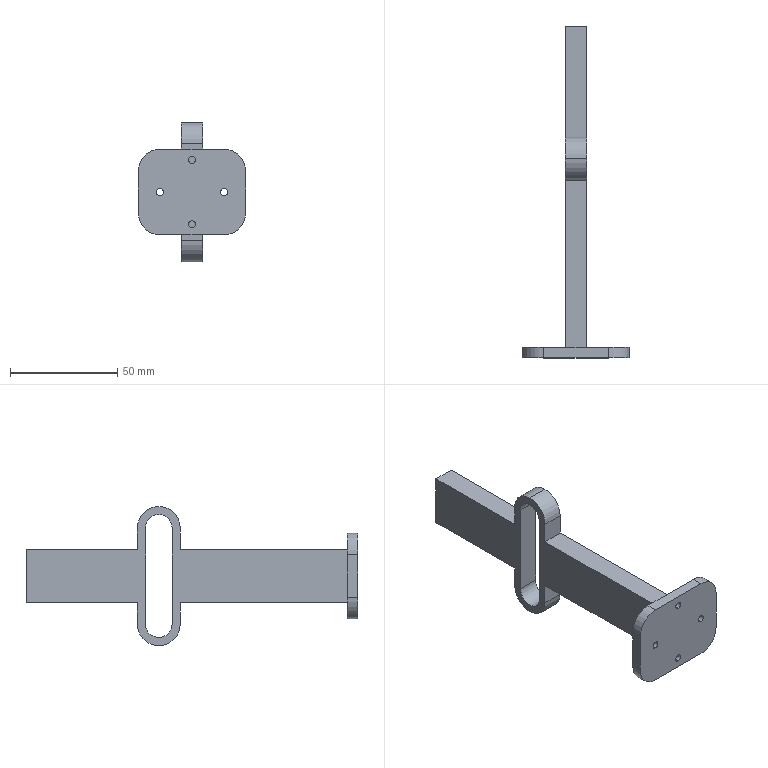Part | SolidWorks | features MirrorStock 1 | 1 solid | 37 faces | box 50 x 155 x 65 mm | volume 47254 mm3 | plane 19 | cylinder 18 | commonest cylinder face diameters 3.3 x8 20 x7 12.4 x3
STEP:
#1=CARTESIAN_POINT('',(15.,2.5,-1.65));
#2=VERTEX_POINT('',#1);
#3=CARTESIAN_POINT('',(15.,2.5,1.65));
#4=VERTEX_POINT('',#3);
#5=CARTESIAN_POINT('',(15.,2.5,0.));
#6=DIRECTION('',(0.,-1.,0.));
#7=DIRECTION('',(0.,0.,-1.));
#8=AXIS2_PLACEMENT_3D('',#5,#6,#7);
#9=CIRCLE('',#8,1.65);
#10=EDGE_CURVE('',#2,#4,#9,.T.);
#11=ORIENTED_EDGE('',*,*,#10,.F.);
#12=CARTESIAN_POINT('',(15.,-2.5,-1.65));
#13=VERTEX_POINT('',#12);
#14=CARTESIAN_POINT('',(15.,32.5,-1.65));
#15=DIRECTION('',(0.,-1.,0.));
#16=VECTOR('',#15,1000.);
#17=LINE('',#14,#16);
#18=EDGE_CURVE('',#2,#13,#17,.T.);
#19=ORIENTED_EDGE('',*,*,#18,.T.);
#20=CARTESIAN_POINT('',(15.,-2.5,1.65));
#21=VERTEX_POINT('',#20);
#22=CARTESIAN_POINT('',(15.,-2.5,0.));
#23=DIRECTION('',(0.,1.,0.));
#24=DIRECTION('',(0.,0.,1.));
#25=AXIS2_PLACEMENT_3D('',#22,#23,#24);
#26=CIRCLE('',#25,1.65);
#27=EDGE_CURVE('',#21,#13,#26,.T.);
#28=ORIENTED_EDGE('',*,*,#27,.F.);
#29=CARTESIAN_POINT('',(15.,32.5,1.65));
#30=DIRECTION('',(0.,-1.,0.));
#31=VECTOR('',#30,1000.);
#32=LINE('',#29,#31);
#33=EDGE_CURVE('',#4,#21,#32,.T.);
#34=ORIENTED_EDGE('',*,*,#33,.F.);
#35=EDGE_LOOP('',(#11,#19,#28,#34));
#36=FACE_OUTER_BOUND('',#35,.T.);
#37=CARTESIAN_POINT('',(15.,32.5,0.));
#38=DIRECTION('',(0.,-1.,0.));
#39=DIRECTION('',(0.,0.,1.));
#40=AXIS2_PLACEMENT_3D('',#37,#38,#39);
#41=CYLINDRICAL_SURFACE('',#40,1.65);
#42=ADVANCED_FACE('',(#36),#41,.F.);
#43=CARTESIAN_POINT('',(0.,2.5,13.35));
#44=VERTEX_POINT('',#43);
#45=CARTESIAN_POINT('',(0.,2.5,16.65));
#46=VERTEX_POINT('',#45);
#47=CARTESIAN_POINT('',(0.,2.5,15.));
#48=DIRECTION('',(0.,-1.,0.));
#49=DIRECTION('',(0.,0.,-1.));
#50=AXIS2_PLACEMENT_3D('',#47,#48,#49);
#51=CIRCLE('',#50,1.65);
#52=EDGE_CURVE('',#44,#46,#51,.T.);
#53=ORIENTED_EDGE('',*,*,#52,.F.);
#54=CARTESIAN_POINT('',(0.,-2.5,13.35));
#55=VERTEX_POINT('',#54);
#56=CARTESIAN_POINT('',(0.,32.5,13.35));
#57=DIRECTION('',(0.,-1.,0.));
#58=VECTOR('',#57,1000.);
#59=LINE('',#56,#58);
#60=EDGE_CURVE('',#44,#55,#59,.T.);
#61=ORIENTED_EDGE('',*,*,#60,.T.);
#62=CARTESIAN_POINT('',(0.,-2.5,16.65));
#63=VERTEX_POINT('',#62);
#64=CARTESIAN_POINT('',(0.,-2.5,15.));
#65=DIRECTION('',(0.,1.,0.));
#66=DIRECTION('',(0.,0.,1.));
#67=AXIS2_PLACEMENT_3D('',#64,#65,#66);
#68=CIRCLE('',#67,1.65);
#69=EDGE_CURVE('',#63,#55,#68,.T.);
#70=ORIENTED_EDGE('',*,*,#69,.F.);
#71=CARTESIAN_POINT('',(0.,32.5,16.65));
#72=DIRECTION('',(0.,-1.,0.));
#73=VECTOR('',#72,1000.);
#74=LINE('',#71,#73);
#75=EDGE_CURVE('',#46,#63,#74,.T.);
#76=ORIENTED_EDGE('',*,*,#75,.F.);
#77=EDGE_LOOP('',(#53,#61,#70,#76));
#78=FACE_OUTER_BOUND('',#77,.T.);
#79=CARTESIAN_POINT('',(0.,32.5,15.));
#80=DIRECTION('',(0.,-1.,0.));
#81=DIRECTION('',(0.,0.,1.));
#82=AXIS2_PLACEMENT_3D('',#79,#80,#81);
#83=CYLINDRICAL_SURFACE('',#82,1.65);
#84=ADVANCED_FACE('',(#78),#83,.F.);
#85=CARTESIAN_POINT('',(0.,2.5,-16.65));
#86=VERTEX_POINT('',#85);
#87=CARTESIAN_POINT('',(0.,2.5,-13.35));
#88=VERTEX_POINT('',#87);
#89=CARTESIAN_POINT('',(0.,2.5,-15.));
#90=DIRECTION('',(0.,-1.,0.));
#91=DIRECTION('',(0.,0.,-1.));
#92=AXIS2_PLACEMENT_3D('',#89,#90,#91);
#93=CIRCLE('',#92,1.65);
#94=EDGE_CURVE('',#86,#88,#93,.T.);
#95=ORIENTED_EDGE('',*,*,#94,.F.);
#96=CARTESIAN_POINT('',(0.,-2.5,-16.65));
#97=VERTEX_POINT('',#96);
#98=CARTESIAN_POINT('',(0.,32.5,-16.65));
#99=DIRECTION('',(0.,-1.,0.));
#100=VECTOR('',#99,1000.);
#101=LINE('',#98,#100);
#102=EDGE_CURVE('',#86,#97,#101,.T.);
#103=ORIENTED_EDGE('',*,*,#102,.T.);
#104=CARTESIAN_POINT('',(0.,-2.5,-13.35));
#105=VERTEX_POINT('',#104);
#106=CARTESIAN_POINT('',(0.,-2.5,-15.));
#107=DIRECTION('',(0.,1.,0.));
#108=DIRECTION('',(0.,0.,1.));
#109=AXIS2_PLACEMENT_3D('',#106,#107,#108);
#110=CIRCLE('',#109,1.65);
#111=EDGE_CURVE('',#105,#97,#110,.T.);
#112=ORIENTED_EDGE('',*,*,#111,.F.);
#113=CARTESIAN_POINT('',(0.,32.5,-13.35));
#114=DIRECTION('',(0.,-1.,0.));
#115=VECTOR('',#114,1000.);
#116=LINE('',#113,#115);
#117=EDGE_CURVE('',#88,#105,#116,.T.);
#118=ORIENTED_EDGE('',*,*,#117,.F.);
#119=EDGE_LOOP('',(#95,#103,#112,#118));
#120=FACE_OUTER_BOUND('',#119,.T.);
#121=CARTESIAN_POINT('',(0.,32.5,-15.));
#122=DIRECTION('',(0.,-1.,0.));
#123=DIRECTION('',(0.,0.,1.));
#124=AXIS2_PLACEMENT_3D('',#121,#122,#123);
#125=CYLINDRICAL_SURFACE('',#124,1.65);
#126=ADVANCED_FACE('',(#120),#125,.F.);
#127=CARTESIAN_POINT('',(-15.,2.5,-1.65));
#128=VERTEX_POINT('',#127);
#129=CARTESIAN_POINT('',(-15.,2.5,1.65));
#130=VERTEX_POINT('',#129);
#131=CARTESIAN_POINT('',(-15.,2.5,0.));
#132=DIRECTION('',(0.,-1.,0.));
#133=DIRECTION('',(0.,0.,-1.));
#134=AXIS2_PLACEMENT_3D('',#131,#132,#133);
#135=CIRCLE('',#134,1.65);
#136=EDGE_CURVE('',#128,#130,#135,.T.);
#137=ORIENTED_EDGE('',*,*,#136,.F.);
#138=CARTESIAN_POINT('',(-15.,-2.5,-1.65));
#139=VERTEX_POINT('',#138);
#140=CARTESIAN_POINT('',(-15.,32.5,-1.65));
#141=DIRECTION('',(0.,-1.,0.));
#142=VECTOR('',#141,1000.);
#143=LINE('',#140,#142);
#144=EDGE_CURVE('',#128,#139,#143,.T.);
#145=ORIENTED_EDGE('',*,*,#144,.T.);
#146=CARTESIAN_POINT('',(-15.,-2.5,1.65));
#147=VERTEX_POINT('',#146);
#148=CARTESIAN_POINT('',(-15.,-2.5,0.));
#149=DIRECTION('',(0.,1.,0.));
#150=DIRECTION('',(0.,0.,1.));
#151=AXIS2_PLACEMENT_3D('',#148,#149,#150);
#152=CIRCLE('',#151,1.65);
#153=EDGE_CURVE('',#147,#139,#152,.T.);
#154=ORIENTED_EDGE('',*,*,#153,.F.);
#155=CARTESIAN_POINT('',(-15.,32.5,1.65));
#156=DIRECTION('',(0.,-1.,0.));
#157=VECTOR('',#156,1000.);
#158=LINE('',#155,#157);
#159=EDGE_CURVE('',#130,#147,#158,.T.);
#160=ORIENTED_EDGE('',*,*,#159,.F.);
#161=EDGE_LOOP('',(#137,#145,#154,#160));
#162=FACE_OUTER_BOUND('',#161,.T.);
#163=CARTESIAN_POINT('',(-15.,32.5,0.));
#164=DIRECTION('',(0.,-1.,0.));
#165=DIRECTION('',(0.,0.,1.));
#166=AXIS2_PLACEMENT_3D('',#163,#164,#165);
#167=CYLINDRICAL_SURFACE('',#166,1.65);
#168=ADVANCED_FACE('',(#162),#167,.F.);
#169=CARTESIAN_POINT('',(-5.,84.3,22.5));
#170=VERTEX_POINT('',#169);
#171=CARTESIAN_POINT('',(-5.,90.5,28.7));
#172=VERTEX_POINT('',#171);
#173=CARTESIAN_POINT('',(-5.,90.5,22.5));
#174=DIRECTION('',(-1.,0.,0.));
#175=DIRECTION('',(0.,0.,1.));
#176=AXIS2_PLACEMENT_3D('',#173,#174,#175);
#177=CIRCLE('',#176,6.2);
#178=EDGE_CURVE('',#170,#172,#177,.T.);
#179=ORIENTED_EDGE('',*,*,#178,.T.);
#180=CARTESIAN_POINT('',(5.,90.5,28.7));
#181=VERTEX_POINT('',#180);
#182=CARTESIAN_POINT('',(-45.,90.5,28.7));
#183=DIRECTION('',(1.,0.,0.));
#184=VECTOR('',#183,1000.);
#185=LINE('',#182,#184);
#186=EDGE_CURVE('',#172,#181,#185,.T.);
#187=ORIENTED_EDGE('',*,*,#186,.T.);
#188=CARTESIAN_POINT('',(5.,84.3,22.5));
#189=VERTEX_POINT('',#188);
#190=CARTESIAN_POINT('',(5.,90.5,22.5));
#191=DIRECTION('',(-1.,0.,0.));
#192=DIRECTION('',(0.,0.,1.));
#193=AXIS2_PLACEMENT_3D('',#190,#191,#192);
#194=CIRCLE('',#193,6.2);
#195=EDGE_CURVE('',#189,#181,#194,.T.);
#196=ORIENTED_EDGE('',*,*,#195,.F.);
#197=CARTESIAN_POINT('',(-45.,84.3,22.5));
#198=DIRECTION('',(1.,0.,0.));
#199=VECTOR('',#198,1000.);
#200=LINE('',#197,#199);
#201=EDGE_CURVE('',#170,#189,#200,.T.);
#202=ORIENTED_EDGE('',*,*,#201,.F.);
#203=EDGE_LOOP('',(#179,#187,#196,#202));
#204=FACE_OUTER_BOUND('',#203,.T.);
#205=CARTESIAN_POINT('',(-45.,90.5,22.5));
#206=DIRECTION('',(1.,0.,0.));
#207=DIRECTION('',(0.,0.,1.));
#208=AXIS2_PLACEMENT_3D('',#205,#206,#207);
#209=CYLINDRICAL_SURFACE('',#208,6.2);
#210=ADVANCED_FACE('',(#204),#209,.F.);
#211=CARTESIAN_POINT('',(-5.,100.5,22.5));
#212=VERTEX_POINT('',#211);
#213=CARTESIAN_POINT('',(-5.,90.5,32.5));
#214=VERTEX_POINT('',#213);
#215=CARTESIAN_POINT('',(-5.,90.5,22.5));
#216=DIRECTION('',(1.,0.,0.));
#217=DIRECTION('',(0.,0.,1.));
#218=AXIS2_PLACEMENT_3D('',#215,#216,#217);
#219=CIRCLE('',#218,10.);
#220=EDGE_CURVE('',#212,#214,#219,.T.);
#221=ORIENTED_EDGE('',*,*,#220,.T.);
#222=CARTESIAN_POINT('',(5.,90.5,32.5));
#223=VERTEX_POINT('',#222);
#224=CARTESIAN_POINT('',(-73.007,90.5,32.5));
#225=DIRECTION('',(1.,0.,0.));
#226=VECTOR('',#225,1000.);
#227=LINE('',#224,#226);
#228=EDGE_CURVE('',#214,#223,#227,.T.);
#229=ORIENTED_EDGE('',*,*,#228,.T.);
#230=CARTESIAN_POINT('',(5.,100.5,22.5));
#231=VERTEX_POINT('',#230);
#232=CARTESIAN_POINT('',(5.,90.5,22.5));
#233=DIRECTION('',(-1.,0.,0.));
#234=DIRECTION('',(0.,0.,1.));
#235=AXIS2_PLACEMENT_3D('',#232,#233,#234);
#236=CIRCLE('',#235,10.);
#237=EDGE_CURVE('',#223,#231,#236,.T.);
#238=ORIENTED_EDGE('',*,*,#237,.T.);
#239=CARTESIAN_POINT('',(-73.007,100.5,22.5));
#240=DIRECTION('',(1.,0.,0.));
#241=VECTOR('',#240,1000.);
#242=LINE('',#239,#241);
#243=EDGE_CURVE('',#212,#231,#242,.T.);
#244=ORIENTED_EDGE('',*,*,#243,.F.);
#245=EDGE_LOOP('',(#221,#229,#238,#244));
#246=FACE_OUTER_BOUND('',#245,.T.);
#247=CARTESIAN_POINT('',(-73.007,90.5,22.5));
#248=DIRECTION('',(1.,0.,0.));
#249=DIRECTION('',(0.,0.,1.));
#250=AXIS2_PLACEMENT_3D('',#247,#248,#249);
#251=CYLINDRICAL_SURFACE('',#250,10.);
#252=ADVANCED_FACE('',(#246),#251,.T.);
#253=CARTESIAN_POINT('',(5.,152.5,12.5));
#254=VERTEX_POINT('',#253);
#255=CARTESIAN_POINT('',(5.,100.5,12.5));
#256=VERTEX_POINT('',#255);
#257=CARTESIAN_POINT('',(5.,152.5,12.5));
#258=DIRECTION('',(0.,-1.,0.));
#259=VECTOR('',#258,1000.);
#260=LINE('',#257,#259);
#261=EDGE_CURVE('',#254,#256,#260,.T.);
#262=ORIENTED_EDGE('',*,*,#261,.F.);
#263=CARTESIAN_POINT('',(-5.,152.5,12.5));
#264=VERTEX_POINT('',#263);
#265=CARTESIAN_POINT('',(-5.,152.5,12.5));
#266=DIRECTION('',(-1.,0.,0.));
#267=VECTOR('',#266,1000.);
#268=LINE('',#265,#267);
#269=EDGE_CURVE('',#254,#264,#268,.T.);
#270=ORIENTED_EDGE('',*,*,#269,.T.);
#271=CARTESIAN_POINT('',(-5.,100.5,12.5));
#272=VERTEX_POINT('',#271);
#273=CARTESIAN_POINT('',(-5.,152.5,12.5));
#274=DIRECTION('',(0.,-1.,0.));
#275=VECTOR('',#274,1000.);
#276=LINE('',#273,#275);
#277=EDGE_CURVE('',#264,#272,#276,.T.);
#278=ORIENTED_EDGE('',*,*,#277,.T.);
#279=CARTESIAN_POINT('',(-5.,100.5,12.5));
#280=DIRECTION('',(-1.,0.,0.));
#281=VECTOR('',#280,1000.);
#282=LINE('',#279,#281);
#283=EDGE_CURVE('',#256,#272,#282,.T.);
#284=ORIENTED_EDGE('',*,*,#283,.F.);
#285=EDGE_LOOP('',(#262,#270,#278,#284));
#286=FACE_OUTER_BOUND('',#285,.T.);
#287=CARTESIAN_POINT('',(-5.,152.5,12.5));
#288=DIRECTION('',(0.,0.,-1.));
#289=DIRECTION('',(1.,0.,0.));
#290=AXIS2_PLACEMENT_3D('',#287,#288,#289);
#291=PLANE('',#290);
#292=ADVANCED_FACE('',(#286),#291,.F.);
#293=CARTESIAN_POINT('',(-5.,152.5,-12.5));
#294=VERTEX_POINT('',#293);
#295=CARTESIAN_POINT('',(-5.,100.5,-12.5));
#296=VERTEX_POINT('',#295);
#297=CARTESIAN_POINT('',(-5.,152.5,-12.5));
#298=DIRECTION('',(0.,-1.,0.));
#299=VECTOR('',#298,1000.);
#300=LINE('',#297,#299);
#301=EDGE_CURVE('',#294,#296,#300,.T.);
#302=ORIENTED_EDGE('',*,*,#301,.F.);
#303=CARTESIAN_POINT('',(5.,152.5,-12.5));
#304=VERTEX_POINT('',#303);
#305=CARTESIAN_POINT('',(-5.,152.5,-12.5));
#306=DIRECTION('',(1.,0.,0.));
#307=VECTOR('',#306,1000.);
#308=LINE('',#305,#307);
#309=EDGE_CURVE('',#294,#304,#308,.T.);
#310=ORIENTED_EDGE('',*,*,#309,.T.);
#311=CARTESIAN_POINT('',(5.,100.5,-12.5));
#312=VERTEX_POINT('',#311);
#313=CARTESIAN_POINT('',(5.,152.5,-12.5));
#314=DIRECTION('',(0.,-1.,0.));
#315=VECTOR('',#314,1000.);
#316=LINE('',#313,#315);
#317=EDGE_CURVE('',#304,#312,#316,.T.);
#318=ORIENTED_EDGE('',*,*,#317,.T.);
#319=CARTESIAN_POINT('',(-5.,100.5,-12.5));
#320=DIRECTION('',(1.,0.,0.));
#321=VECTOR('',#320,1000.);
#322=LINE('',#319,#321);
#323=EDGE_CURVE('',#296,#312,#322,.T.);
#324=ORIENTED_EDGE('',*,*,#323,.F.);
#325=EDGE_LOOP('',(#302,#310,#318,#324));
#326=FACE_OUTER_BOUND('',#325,.T.);
#327=CARTESIAN_POINT('',(-5.,152.5,-12.5));
#328=DIRECTION('',(0.,0.,1.));
#329=DIRECTION('',(-1.,0.,0.));
#330=AXIS2_PLACEMENT_3D('',#327,#328,#329);
#331=PLANE('',#330);
#332=ADVANCED_FACE('',(#326),#331,.F.);
#333=ORIENTED_EDGE('',*,*,#27,.T.);
#334=CARTESIAN_POINT('',(15.,-2.5,0.));
#335=DIRECTION('',(0.,1.,0.));
#336=DIRECTION('',(0.,0.,1.));
#337=AXIS2_PLACEMENT_3D('',#334,#335,#336);
#338=CIRCLE('',#337,1.65);
#339=EDGE_CURVE('',#13,#21,#338,.T.);
#340=ORIENTED_EDGE('',*,*,#339,.T.);
#341=EDGE_LOOP('',(#333,#340));
#342=FACE_BOUND('',#341,.T.);
#343=ORIENTED_EDGE('',*,*,#69,.T.);
#344=CARTESIAN_POINT('',(0.,-2.5,15.));
#345=DIRECTION('',(0.,1.,0.));
#346=DIRECTION('',(0.,0.,1.));
#347=AXIS2_PLACEMENT_3D('',#344,#345,#346);
#348=CIRCLE('',#347,1.65);
#349=EDGE_CURVE('',#55,#63,#348,.T.);
#350=ORIENTED_EDGE('',*,*,#349,.T.);
#351=EDGE_LOOP('',(#343,#350));
#352=FACE_BOUND('',#351,.T.);
#353=ORIENTED_EDGE('',*,*,#111,.T.);
#354=CARTESIAN_POINT('',(0.,-2.5,-15.));
#355=DIRECTION('',(0.,1.,0.));
#356=DIRECTION('',(0.,0.,1.));
#357=AXIS2_PLACEMENT_3D('',#354,#355,#356);
#358=CIRCLE('',#357,1.65);
#359=EDGE_CURVE('',#97,#105,#358,.T.);
#360=ORIENTED_EDGE('',*,*,#359,.T.);
#361=EDGE_LOOP('',(#353,#360));
#362=FACE_BOUND('',#361,.T.);
#363=ORIENTED_EDGE('',*,*,#153,.T.);
#364=CARTESIAN_POINT('',(-15.,-2.5,0.));
#365=DIRECTION('',(0.,1.,0.));
#366=DIRECTION('',(0.,0.,1.));
#367=AXIS2_PLACEMENT_3D('',#364,#365,#366);
#368=CIRCLE('',#367,1.65);
#369=EDGE_CURVE('',#139,#147,#368,.T.);
#370=ORIENTED_EDGE('',*,*,#369,.T.);
#371=EDGE_LOOP('',(#363,#370));
#372=FACE_BOUND('',#371,.T.);
#373=CARTESIAN_POINT('',(-25.,-2.5,-10.));
#374=VERTEX_POINT('',#373);
#375=CARTESIAN_POINT('',(-25.,-2.5,10.));
#376=VERTEX_POINT('',#375);
#377=CARTESIAN_POINT('',(-25.,-2.5,-20.));
#378=DIRECTION('',(0.,0.,1.));
#379=VECTOR('',#378,1000.);
#380=LINE('',#377,#379);
#381=EDGE_CURVE('',#374,#376,#380,.T.);
#382=ORIENTED_EDGE('',*,*,#381,.F.);
#383=CARTESIAN_POINT('',(-15.,-2.5,-20.));
#384=VERTEX_POINT('',#383);
#385=CARTESIAN_POINT('',(-15.,-2.5,-10.));
#386=DIRECTION('',(0.,1.,0.));
#387=DIRECTION('',(0.,0.,-1.));
#388=AXIS2_PLACEMENT_3D('',#385,#386,#387);
#389=CIRCLE('',#388,10.);
#390=EDGE_CURVE('',#384,#374,#389,.T.);
#391=ORIENTED_EDGE('',*,*,#390,.F.);
#392=CARTESIAN_POINT('',(15.,-2.5,-20.));
#393=VERTEX_POINT('',#392);
#394=CARTESIAN_POINT('',(0.,-2.5,-20.));
#395=DIRECTION('',(1.,0.,0.));
#396=VECTOR('',#395,1000.);
#397=LINE('',#394,#396);
#398=EDGE_CURVE('',#384,#393,#397,.T.);
#399=ORIENTED_EDGE('',*,*,#398,.T.);
#400=CARTESIAN_POINT('',(25.,-2.5,-10.));
#401=VERTEX_POINT('',#400);
#402=CARTESIAN_POINT('',(15.,-2.5,-10.));
#403=DIRECTION('',(0.,1.,0.));
#404=DIRECTION('',(0.,0.,-1.));
#405=AXIS2_PLACEMENT_3D('',#402,#403,#404);
#406=CIRCLE('',#405,10.);
#407=EDGE_CURVE('',#401,#393,#406,.T.);
#408=ORIENTED_EDGE('',*,*,#407,.F.);
#409=CARTESIAN_POINT('',(25.,-2.5,10.));
#410=VERTEX_POINT('',#409);
#411=CARTESIAN_POINT('',(25.,-2.5,-20.));
#412=DIRECTION('',(0.,0.,1.));
#413=VECTOR('',#412,1000.);
#414=LINE('',#411,#413);
#415=EDGE_CURVE('',#401,#410,#414,.T.);
#416=ORIENTED_EDGE('',*,*,#415,.T.);
#417=CARTESIAN_POINT('',(15.,-2.5,20.));
#418=VERTEX_POINT('',#417);
#419=CARTESIAN_POINT('',(15.,-2.5,10.));
#420=DIRECTION('',(0.,1.,0.));
#421=DIRECTION('',(0.,0.,-1.));
#422=AXIS2_PLACEMENT_3D('',#419,#420,#421);
#423=CIRCLE('',#422,10.);
#424=EDGE_CURVE('',#418,#410,#423,.T.);
#425=ORIENTED_EDGE('',*,*,#424,.F.);
#426=CARTESIAN_POINT('',(-15.,-2.5,20.));
#427=VERTEX_POINT('',#426);
#428=CARTESIAN_POINT('',(0.,-2.5,20.));
#429=DIRECTION('',(1.,0.,0.));
#430=VECTOR('',#429,1000.);
#431=LINE('',#428,#430);
#432=EDGE_CURVE('',#427,#418,#431,.T.);
#433=ORIENTED_EDGE('',*,*,#432,.F.);
#434=CARTESIAN_POINT('',(-15.,-2.5,10.));
#435=DIRECTION('',(0.,1.,0.));
#436=DIRECTION('',(0.,0.,-1.));
#437=AXIS2_PLACEMENT_3D('',#434,#435,#436);
#438=CIRCLE('',#437,10.);
#439=EDGE_CURVE('',#376,#427,#438,.T.);
#440=ORIENTED_EDGE('',*,*,#439,.F.);
#441=EDGE_LOOP('',(#382,#391,#399,#408,#416,#425,#433,#440));
#442=FACE_OUTER_BOUND('',#441,.T.);
#443=CARTESIAN_POINT('',(0.,-2.5,-20.));
#444=DIRECTION('',(0.,1.,0.));
#445=DIRECTION('',(0.,0.,-1.));
#446=AXIS2_PLACEMENT_3D('',#443,#444,#445);
#447=PLANE('',#446);
#448=ADVANCED_FACE('',(#342,#352,#362,#372,#442),#447,.F.);
#449=ORIENTED_EDGE('',*,*,#415,.F.);
#450=CARTESIAN_POINT('',(25.,2.5,-10.));
#451=VERTEX_POINT('',#450);
#452=CARTESIAN_POINT('',(25.,-2.5,-10.));
#453=DIRECTION('',(0.,-1.,0.));
#454=VECTOR('',#453,1000.);
#455=LINE('',#452,#454);
#456=EDGE_CURVE('',#451,#401,#455,.T.);
#457=ORIENTED_EDGE('',*,*,#456,.F.);
#458=CARTESIAN_POINT('',(25.,2.5,10.));
#459=VERTEX_POINT('',#458);
#460=CARTESIAN_POINT('',(25.,2.5,-20.));
#461=DIRECTION('',(0.,0.,1.));
#462=VECTOR('',#461,1000.);
#463=LINE('',#460,#462);
#464=EDGE_CURVE('',#451,#459,#463,.T.);
#465=ORIENTED_EDGE('',*,*,#464,.T.);
#466=CARTESIAN_POINT('',(25.,0.,10.));
#467=DIRECTION('',(0.,1.,0.));
#468=VECTOR('',#467,1000.);
#469=LINE('',#466,#468);
#470=EDGE_CURVE('',#410,#459,#469,.T.);
#471=ORIENTED_EDGE('',*,*,#470,.F.);
#472=EDGE_LOOP('',(#449,#457,#465,#471));
#473=FACE_OUTER_BOUND('',#472,.T.);
#474=CARTESIAN_POINT('',(25.,0.,-20.));
#475=DIRECTION('',(-1.,0.,0.));
#476=DIRECTION('',(0.,0.,-1.));
#477=AXIS2_PLACEMENT_3D('',#474,#475,#476);
#478=PLANE('',#477);
#479=ADVANCED_FACE('',(#473),#478,.F.);
#480=CARTESIAN_POINT('',(15.,2.5,0.));
#481=DIRECTION('',(0.,-1.,0.));
#482=DIRECTION('',(0.,0.,-1.));
#483=AXIS2_PLACEMENT_3D('',#480,#481,#482);
#484=CIRCLE('',#483,1.65);
#485=EDGE_CURVE('',#4,#2,#484,.T.);
#486=ORIENTED_EDGE('',*,*,#485,.T.);
#487=ORIENTED_EDGE('',*,*,#10,.T.);
#488=EDGE_LOOP('',(#486,#487));
#489=FACE_BOUND('',#488,.T.);
#490=CARTESIAN_POINT('',(0.,2.5,15.));
#491=DIRECTION('',(0.,-1.,0.));
#492=DIRECTION('',(0.,0.,-1.));
#493=AXIS2_PLACEMENT_3D('',#490,#491,#492);
#494=CIRCLE('',#493,1.65);
#495=EDGE_CURVE('',#46,#44,#494,.T.);
#496=ORIENTED_EDGE('',*,*,#495,.T.);
#497=ORIENTED_EDGE('',*,*,#52,.T.);
#498=EDGE_LOOP('',(#496,#497));
#499=FACE_BOUND('',#498,.T.);
#500=CARTESIAN_POINT('',(0.,2.5,-15.));
#501=DIRECTION('',(0.,-1.,0.));
#502=DIRECTION('',(0.,0.,-1.));
#503=AXIS2_PLACEMENT_3D('',#500,#501,#502);
#504=CIRCLE('',#503,1.65);
#505=EDGE_CURVE('',#88,#86,#504,.T.);
#506=ORIENTED_EDGE('',*,*,#505,.T.);
#507=ORIENTED_EDGE('',*,*,#94,.T.);
#508=EDGE_LOOP('',(#506,#507));
#509=FACE_BOUND('',#508,.T.);
#510=CARTESIAN_POINT('',(-15.,2.5,0.));
#511=DIRECTION('',(0.,-1.,0.));
#512=DIRECTION('',(0.,0.,-1.));
#513=AXIS2_PLACEMENT_3D('',#510,#511,#512);
#514=CIRCLE('',#513,1.65);
#515=EDGE_CURVE('',#130,#128,#514,.T.);
#516=ORIENTED_EDGE('',*,*,#515,.T.);
#517=ORIENTED_EDGE('',*,*,#136,.T.);
#518=EDGE_LOOP('',(#516,#517));
#519=FACE_BOUND('',#518,.T.);
#520=CARTESIAN_POINT('',(5.,2.5,-12.5));
#521=VERTEX_POINT('',#520);
#522=CARTESIAN_POINT('',(5.,2.5,12.5));
#523=VERTEX_POINT('',#522);
#524=CARTESIAN_POINT('',(5.,2.5,-12.5));
#525=DIRECTION('',(0.,0.,1.));
#526=VECTOR('',#525,1000.);
#527=LINE('',#524,#526);
#528=EDGE_CURVE('',#521,#523,#527,.T.);
#529=ORIENTED_EDGE('',*,*,#528,.T.);
#530=CARTESIAN_POINT('',(-5.,2.5,12.5));
#531=VERTEX_POINT('',#530);
#532=CARTESIAN_POINT('',(-5.,2.5,12.5));
#533=DIRECTION('',(-1.,0.,0.));
#534=VECTOR('',#533,1000.);
#535=LINE('',#532,#534);
#536=EDGE_CURVE('',#523,#531,#535,.T.);
#537=ORIENTED_EDGE('',*,*,#536,.T.);
#538=CARTESIAN_POINT('',(-5.,2.5,-12.5));
#539=VERTEX_POINT('',#538);
#540=CARTESIAN_POINT('',(-5.,2.5,-12.5));
#541=DIRECTION('',(0.,0.,-1.));
#542=VECTOR('',#541,1000.);
#543=LINE('',#540,#542);
#544=EDGE_CURVE('',#531,#539,#543,.T.);
#545=ORIENTED_EDGE('',*,*,#544,.T.);
#546=CARTESIAN_POINT('',(-5.,2.5,-12.5));
#547=DIRECTION('',(1.,0.,0.));
#548=VECTOR('',#547,1000.);
#549=LINE('',#546,#548);
#550=EDGE_CURVE('',#539,#521,#549,.T.);
#551=ORIENTED_EDGE('',*,*,#550,.T.);
#552=EDGE_LOOP('',(#529,#537,#545,#551));
#553=FACE_BOUND('',#552,.T.);
#554=CARTESIAN_POINT('',(-15.,2.5,20.));
#555=VERTEX_POINT('',#554);
#556=CARTESIAN_POINT('',(15.,2.5,20.));
#557=VERTEX_POINT('',#556);
#558=CARTESIAN_POINT('',(0.,2.5,20.));
#559=DIRECTION('',(1.,0.,0.));
#560=VECTOR('',#559,1000.);
#561=LINE('',#558,#560);
#562=EDGE_CURVE('',#555,#557,#561,.T.);
#563=ORIENTED_EDGE('',*,*,#562,.T.);
#564=CARTESIAN_POINT('',(15.,2.5,10.));
#565=DIRECTION('',(0.,-1.,0.));
#566=DIRECTION('',(0.,0.,-1.));
#567=AXIS2_PLACEMENT_3D('',#564,#565,#566);
#568=CIRCLE('',#567,10.);
#569=EDGE_CURVE('',#459,#557,#568,.T.);
#570=ORIENTED_EDGE('',*,*,#569,.F.);
#571=ORIENTED_EDGE('',*,*,#464,.F.);
#572=CARTESIAN_POINT('',(15.,2.5,-20.));
#573=VERTEX_POINT('',#572);
#574=CARTESIAN_POINT('',(15.,2.5,-10.));
#575=DIRECTION('',(0.,-1.,0.));
#576=DIRECTION('',(0.,0.,-1.));
#577=AXIS2_PLACEMENT_3D('',#574,#575,#576);
#578=CIRCLE('',#577,10.);
#579=EDGE_CURVE('',#573,#451,#578,.T.);
#580=ORIENTED_EDGE('',*,*,#579,.F.);
#581=CARTESIAN_POINT('',(-15.,2.5,-20.));
#582=VERTEX_POINT('',#581);
#583=CARTESIAN_POINT('',(0.,2.5,-20.));
#584=DIRECTION('',(1.,0.,0.));
#585=VECTOR('',#584,1000.);
#586=LINE('',#583,#585);
#587=EDGE_CURVE('',#582,#573,#586,.T.);
#588=ORIENTED_EDGE('',*,*,#587,.F.);
#589=CARTESIAN_POINT('',(-25.,2.5,-10.));
#590=VERTEX_POINT('',#589);
#591=CARTESIAN_POINT('',(-15.,2.5,-10.));
#592=DIRECTION('',(0.,-1.,0.));
#593=DIRECTION('',(0.,0.,-1.));
#594=AXIS2_PLACEMENT_3D('',#591,#592,#593);
#595=CIRCLE('',#594,10.);
#596=EDGE_CURVE('',#590,#582,#595,.T.);
#597=ORIENTED_EDGE('',*,*,#596,.F.);
#598=CARTESIAN_POINT('',(-25.,2.5,10.));
#599=VERTEX_POINT('',#598);
#600=CARTESIAN_POINT('',(-25.,2.5,-20.));
#601=DIRECTION('',(0.,0.,1.));
#602=VECTOR('',#601,1000.);
#603=LINE('',#600,#602);
#604=EDGE_CURVE('',#590,#599,#603,.T.);
#605=ORIENTED_EDGE('',*,*,#604,.T.);
#606=CARTESIAN_POINT('',(-15.,2.5,10.));
#607=DIRECTION('',(0.,-1.,0.));
#608=DIRECTION('',(0.,0.,-1.));
#609=AXIS2_PLACEMENT_3D('',#606,#607,#608);
#610=CIRCLE('',#609,10.);
#611=EDGE_CURVE('',#555,#599,#610,.T.);
#612=ORIENTED_EDGE('',*,*,#611,.F.);
#613=EDGE_LOOP('',(#563,#570,#571,#580,#588,#597,#605,#612));
#614=FACE_OUTER_BOUND('',#613,.T.);
#615=CARTESIAN_POINT('',(0.,2.5,-20.));
#616=DIRECTION('',(0.,1.,0.));
#617=DIRECTION('',(0.,0.,-1.));
#618=AXIS2_PLACEMENT_3D('',#615,#616,#617);
#619=PLANE('',#618);
#620=ADVANCED_FACE('',(#489,#499,#509,#519,#553,#614),#619,.T.);
#621=ORIENTED_EDGE('',*,*,#604,.F.);
#622=CARTESIAN_POINT('',(-25.,0.,-10.));
#623=DIRECTION('',(0.,1.,0.));
#624=VECTOR('',#623,1000.);
#625=LINE('',#622,#624);
#626=EDGE_CURVE('',#374,#590,#625,.T.);
#627=ORIENTED_EDGE('',*,*,#626,.F.);
#628=ORIENTED_EDGE('',*,*,#381,.T.);
#629=CARTESIAN_POINT('',(-25.,-2.5,10.));
#630=DIRECTION('',(0.,-1.,0.));
#631=VECTOR('',#630,1000.);
#632=LINE('',#629,#631);
#633=EDGE_CURVE('',#599,#376,#632,.T.);
#634=ORIENTED_EDGE('',*,*,#633,.F.);
#635=EDGE_LOOP('',(#621,#627,#628,#634));
#636=FACE_OUTER_BOUND('',#635,.T.);
#637=CARTESIAN_POINT('',(-25.,0.,-20.));
#638=DIRECTION('',(-1.,0.,0.));
#639=DIRECTION('',(0.,0.,-1.));
#640=AXIS2_PLACEMENT_3D('',#637,#638,#639);
#641=PLANE('',#640);
#642=ADVANCED_FACE('',(#636),#641,.T.);
#643=ORIENTED_EDGE('',*,*,#398,.F.);
#644=CARTESIAN_POINT('',(-15.,0.,-20.));
#645=DIRECTION('',(0.,-1.,0.));
#646=VECTOR('',#645,1000.);
#647=LINE('',#644,#646);
#648=EDGE_CURVE('',#582,#384,#647,.T.);
#649=ORIENTED_EDGE('',*,*,#648,.F.);
#650=ORIENTED_EDGE('',*,*,#587,.T.);
#651=CARTESIAN_POINT('',(15.,2.5,-20.));
#652=DIRECTION('',(0.,1.,0.));
#653=VECTOR('',#652,1000.);
#654=LINE('',#651,#653);
#655=EDGE_CURVE('',#393,#573,#654,.T.);
#656=ORIENTED_EDGE('',*,*,#655,.F.);
#657=EDGE_LOOP('',(#643,#649,#650,#656));
#658=FACE_OUTER_BOUND('',#657,.T.);
#659=CARTESIAN_POINT('',(0.,0.,-20.));
#660=DIRECTION('',(0.,0.,-1.));
#661=DIRECTION('',(1.,0.,0.));
#662=AXIS2_PLACEMENT_3D('',#659,#660,#661);
#663=PLANE('',#662);
#664=ADVANCED_FACE('',(#658),#663,.T.);
#665=ORIENTED_EDGE('',*,*,#432,.T.);
#666=CARTESIAN_POINT('',(15.,0.,20.));
#667=DIRECTION('',(0.,-1.,0.));
#668=VECTOR('',#667,1000.);
#669=LINE('',#666,#668);
#670=EDGE_CURVE('',#557,#418,#669,.T.);
#671=ORIENTED_EDGE('',*,*,#670,.F.);
#672=ORIENTED_EDGE('',*,*,#562,.F.);
#673=CARTESIAN_POINT('',(-15.,2.5,20.));
#674=DIRECTION('',(0.,1.,0.));
#675=VECTOR('',#674,1000.);
#676=LINE('',#673,#675);
#677=EDGE_CURVE('',#427,#555,#676,.T.);
#678=ORIENTED_EDGE('',*,*,#677,.F.);
#679=EDGE_LOOP('',(#665,#671,#672,#678));
#680=FACE_OUTER_BOUND('',#679,.T.);
#681=CARTESIAN_POINT('',(0.,0.,20.));
#682=DIRECTION('',(0.,0.,-1.));
#683=DIRECTION('',(1.,0.,0.));
#684=AXIS2_PLACEMENT_3D('',#681,#682,#683);
#685=PLANE('',#684);
#686=ADVANCED_FACE('',(#680),#685,.F.);
#687=CARTESIAN_POINT('',(5.,96.7,-22.5));
#688=VERTEX_POINT('',#687);
#689=CARTESIAN_POINT('',(5.,84.3,-22.5));
#690=VERTEX_POINT('',#689);
#691=CARTESIAN_POINT('',(5.,90.5,-22.5));
#692=DIRECTION('',(-1.,0.,0.));
#693=DIRECTION('',(0.,0.,1.));
#694=AXIS2_PLACEMENT_3D('',#691,#692,#693);
#695=CIRCLE('',#694,6.2);
#696=EDGE_CURVE('',#688,#690,#695,.T.);
#697=ORIENTED_EDGE('',*,*,#696,.T.);
#698=CARTESIAN_POINT('',(5.,84.3,0.));
#699=DIRECTION('',(0.,0.,1.));
#700=VECTOR('',#699,1000.);
#701=LINE('',#698,#700);
#702=EDGE_CURVE('',#690,#189,#701,.T.);
#703=ORIENTED_EDGE('',*,*,#702,.T.);
#704=ORIENTED_EDGE('',*,*,#195,.T.);
#705=CARTESIAN_POINT('',(5.,96.7,22.5));
#706=VERTEX_POINT('',#705);
#707=CARTESIAN_POINT('',(5.,90.5,22.5));
#708=DIRECTION('',(-1.,0.,0.));
#709=DIRECTION('',(0.,0.,1.));
#710=AXIS2_PLACEMENT_3D('',#707,#708,#709);
#711=CIRCLE('',#710,6.2);
#712=EDGE_CURVE('',#181,#706,#711,.T.);
#713=ORIENTED_EDGE('',*,*,#712,.T.);
#714=CARTESIAN_POINT('',(5.,96.7,0.));
#715=DIRECTION('',(0.,0.,-1.));
#716=VECTOR('',#715,1000.);
#717=LINE('',#714,#716);
#718=EDGE_CURVE('',#706,#688,#717,.T.);
#719=ORIENTED_EDGE('',*,*,#718,.T.);
#720=EDGE_LOOP('',(#697,#703,#704,#713,#719));
#721=FACE_BOUND('',#720,.T.);
#722=CARTESIAN_POINT('',(5.,80.5,12.5));
#723=VERTEX_POINT('',#722);
#724=CARTESIAN_POINT('',(5.,152.5,12.5));
#725=DIRECTION('',(0.,-1.,0.));
#726=VECTOR('',#725,1000.);
#727=LINE('',#724,#726);
#728=EDGE_CURVE('',#723,#523,#727,.T.);
#729=ORIENTED_EDGE('',*,*,#728,.T.);
#730=ORIENTED_EDGE('',*,*,#528,.F.);
#731=CARTESIAN_POINT('',(5.,80.5,-12.5));
#732=VERTEX_POINT('',#731);
#733=CARTESIAN_POINT('',(5.,152.5,-12.5));
#734=DIRECTION('',(0.,-1.,0.));
#735=VECTOR('',#734,1000.);
#736=LINE('',#733,#735);
#737=EDGE_CURVE('',#732,#521,#736,.T.);
#738=ORIENTED_EDGE('',*,*,#737,.F.);
#739=CARTESIAN_POINT('',(5.,80.5,-22.5));
#740=VERTEX_POINT('',#739);
#741=CARTESIAN_POINT('',(5.,80.5,-22.5));
#742=DIRECTION('',(0.,0.,1.));
#743=VECTOR('',#742,1000.);
#744=LINE('',#741,#743);
#745=EDGE_CURVE('',#740,#732,#744,.T.);
#746=ORIENTED_EDGE('',*,*,#745,.F.);
#747=CARTESIAN_POINT('',(5.,100.5,-22.5));
#748=VERTEX_POINT('',#747);
#749=CARTESIAN_POINT('',(5.,90.5,-22.5));
#750=DIRECTION('',(-1.,0.,0.));
#751=DIRECTION('',(0.,0.,1.));
#752=AXIS2_PLACEMENT_3D('',#749,#750,#751);
#753=CIRCLE('',#752,10.);
#754=EDGE_CURVE('',#748,#740,#753,.T.);
#755=ORIENTED_EDGE('',*,*,#754,.F.);
#756=CARTESIAN_POINT('',(5.,100.5,-22.5));
#757=DIRECTION('',(0.,0.,-1.));
#758=VECTOR('',#757,1000.);
#759=LINE('',#756,#758);
#760=EDGE_CURVE('',#312,#748,#759,.T.);
#761=ORIENTED_EDGE('',*,*,#760,.F.);
#762=ORIENTED_EDGE('',*,*,#317,.F.);
#763=CARTESIAN_POINT('',(5.,152.5,-12.5));
#764=DIRECTION('',(0.,0.,1.));
#765=VECTOR('',#764,1000.);
#766=LINE('',#763,#765);
#767=EDGE_CURVE('',#304,#254,#766,.T.);
#768=ORIENTED_EDGE('',*,*,#767,.T.);
#769=ORIENTED_EDGE('',*,*,#261,.T.);
#770=CARTESIAN_POINT('',(5.,100.5,-22.5));
#771=DIRECTION('',(0.,0.,-1.));
#772=VECTOR('',#771,1000.);
#773=LINE('',#770,#772);
#774=EDGE_CURVE('',#231,#256,#773,.T.);
#775=ORIENTED_EDGE('',*,*,#774,.F.);
#776=ORIENTED_EDGE('',*,*,#237,.F.);
#777=CARTESIAN_POINT('',(5.,80.5,22.5));
#778=VERTEX_POINT('',#777);
#779=CARTESIAN_POINT('',(5.,90.5,22.5));
#780=DIRECTION('',(-1.,0.,0.));
#781=DIRECTION('',(0.,0.,1.));
#782=AXIS2_PLACEMENT_3D('',#779,#780,#781);
#783=CIRCLE('',#782,10.);
#784=EDGE_CURVE('',#778,#223,#783,.T.);
#785=ORIENTED_EDGE('',*,*,#784,.F.);
#786=CARTESIAN_POINT('',(5.,80.5,-22.5));
#787=DIRECTION('',(0.,0.,1.));
#788=VECTOR('',#787,1000.);
#789=LINE('',#786,#788);
#790=EDGE_CURVE('',#723,#778,#789,.T.);
#791=ORIENTED_EDGE('',*,*,#790,.F.);
#792=EDGE_LOOP('',(#729,#730,#738,#746,#755,#761,#762,#768,#769,#775,#776,#785,#791));
#793=FACE_OUTER_BOUND('',#792,.T.);
#794=CARTESIAN_POINT('',(5.,152.5,-12.5));
#795=DIRECTION('',(-1.,0.,0.));
#796=DIRECTION('',(0.,0.,-1.));
#797=AXIS2_PLACEMENT_3D('',#794,#795,#796);
#798=PLANE('',#797);
#799=ADVANCED_FACE('',(#721,#793),#798,.F.);
#800=CARTESIAN_POINT('',(-5.,80.5,12.5));
#801=VERTEX_POINT('',#800);
#802=CARTESIAN_POINT('',(-5.,152.5,12.5));
#803=DIRECTION('',(0.,-1.,0.));
#804=VECTOR('',#803,1000.);
#805=LINE('',#802,#804);
#806=EDGE_CURVE('',#801,#531,#805,.T.);
#807=ORIENTED_EDGE('',*,*,#806,.T.);
#808=ORIENTED_EDGE('',*,*,#536,.F.);
#809=ORIENTED_EDGE('',*,*,#728,.F.);
#810=CARTESIAN_POINT('',(-5.,80.5,12.5));
#811=DIRECTION('',(1.,0.,0.));
#812=VECTOR('',#811,1000.);
#813=LINE('',#810,#812);
#814=EDGE_CURVE('',#801,#723,#813,.T.);
#815=ORIENTED_EDGE('',*,*,#814,.F.);
#816=EDGE_LOOP('',(#807,#808,#809,#815));
#817=FACE_OUTER_BOUND('',#816,.T.);
#818=CARTESIAN_POINT('',(-5.,152.5,12.5));
#819=DIRECTION('',(0.,0.,-1.));
#820=DIRECTION('',(1.,0.,0.));
#821=AXIS2_PLACEMENT_3D('',#818,#819,#820);
#822=PLANE('',#821);
#823=ADVANCED_FACE('',(#817),#822,.F.);
#824=ORIENTED_EDGE('',*,*,#178,.F.);
#825=CARTESIAN_POINT('',(-5.,84.3,-22.5));
#826=VERTEX_POINT('',#825);
#827=CARTESIAN_POINT('',(-5.,84.3,-12.5));
#828=DIRECTION('',(0.,0.,1.));
#829=VECTOR('',#828,1000.);
#830=LINE('',#827,#829);
#831=EDGE_CURVE('',#826,#170,#830,.T.);
#832=ORIENTED_EDGE('',*,*,#831,.F.);
#833=CARTESIAN_POINT('',(-5.,96.7,-22.5));
#834=VERTEX_POINT('',#833);
#835=CARTESIAN_POINT('',(-5.,90.5,-22.5));
#836=DIRECTION('',(-1.,0.,0.));
#837=DIRECTION('',(0.,0.,1.));
#838=AXIS2_PLACEMENT_3D('',#835,#836,#837);
#839=CIRCLE('',#838,6.2);
#840=EDGE_CURVE('',#834,#826,#839,.T.);
#841=ORIENTED_EDGE('',*,*,#840,.F.);
#842=CARTESIAN_POINT('',(-5.,96.7,22.5));
#843=VERTEX_POINT('',#842);
#844=CARTESIAN_POINT('',(-5.,96.7,-12.5));
#845=DIRECTION('',(0.,0.,-1.));
#846=VECTOR('',#845,1000.);
#847=LINE('',#844,#846);
#848=EDGE_CURVE('',#843,#834,#847,.T.);
#849=ORIENTED_EDGE('',*,*,#848,.F.);
#850=CARTESIAN_POINT('',(-5.,90.5,22.5));
#851=DIRECTION('',(-1.,0.,0.));
#852=DIRECTION('',(0.,0.,1.));
#853=AXIS2_PLACEMENT_3D('',#850,#851,#852);
#854=CIRCLE('',#853,6.2);
#855=EDGE_CURVE('',#172,#843,#854,.T.);
#856=ORIENTED_EDGE('',*,*,#855,.F.);
#857=EDGE_LOOP('',(#824,#832,#841,#849,#856));
#858=FACE_BOUND('',#857,.T.);
#859=CARTESIAN_POINT('',(-5.,80.5,-12.5));
#860=VERTEX_POINT('',#859);
#861=CARTESIAN_POINT('',(-5.,152.5,-12.5));
#862=DIRECTION('',(0.,-1.,0.));
#863=VECTOR('',#862,1000.);
#864=LINE('',#861,#863);
#865=EDGE_CURVE('',#860,#539,#864,.T.);
#866=ORIENTED_EDGE('',*,*,#865,.T.);
#867=ORIENTED_EDGE('',*,*,#544,.F.);
#868=ORIENTED_EDGE('',*,*,#806,.F.);
#869=CARTESIAN_POINT('',(-5.,80.5,22.5));
#870=VERTEX_POINT('',#869);
#871=CARTESIAN_POINT('',(-5.,80.5,-22.5));
#872=DIRECTION('',(0.,0.,-1.));
#873=VECTOR('',#872,1000.);
#874=LINE('',#871,#873);
#875=EDGE_CURVE('',#870,#801,#874,.T.);
#876=ORIENTED_EDGE('',*,*,#875,.F.);
#877=CARTESIAN_POINT('',(-5.,90.5,22.5));
#878=DIRECTION('',(1.,0.,0.));
#879=DIRECTION('',(0.,0.,1.));
#880=AXIS2_PLACEMENT_3D('',#877,#878,#879);
#881=CIRCLE('',#880,10.);
#882=EDGE_CURVE('',#214,#870,#881,.T.);
#883=ORIENTED_EDGE('',*,*,#882,.F.);
#884=ORIENTED_EDGE('',*,*,#220,.F.);
#885=CARTESIAN_POINT('',(-5.,100.5,-22.5));
#886=DIRECTION('',(0.,0.,1.));
#887=VECTOR('',#886,1000.);
#888=LINE('',#885,#887);
#889=EDGE_CURVE('',#272,#212,#888,.T.);
#890=ORIENTED_EDGE('',*,*,#889,.F.);
#891=ORIENTED_EDGE('',*,*,#277,.F.);
#892=CARTESIAN_POINT('',(-5.,152.5,-12.5));
#893=DIRECTION('',(0.,0.,-1.));
#894=VECTOR('',#893,1000.);
#895=LINE('',#892,#894);
#896=EDGE_CURVE('',#264,#294,#895,.T.);
#897=ORIENTED_EDGE('',*,*,#896,.T.);
#898=ORIENTED_EDGE('',*,*,#301,.T.);
#899=CARTESIAN_POINT('',(-5.,100.5,-22.5));
#900=VERTEX_POINT('',#899);
#901=CARTESIAN_POINT('',(-5.,100.5,-22.5));
#902=DIRECTION('',(0.,0.,1.));
#903=VECTOR('',#902,1000.);
#904=LINE('',#901,#903);
#905=EDGE_CURVE('',#900,#296,#904,.T.);
#906=ORIENTED_EDGE('',*,*,#905,.F.);
#907=CARTESIAN_POINT('',(-5.,80.5,-22.5));
#908=VERTEX_POINT('',#907);
#909=CARTESIAN_POINT('',(-5.,90.5,-22.5));
#910=DIRECTION('',(1.,0.,0.));
#911=DIRECTION('',(0.,0.,1.));
#912=AXIS2_PLACEMENT_3D('',#909,#910,#911);
#913=CIRCLE('',#912,10.);
#914=EDGE_CURVE('',#908,#900,#913,.T.);
#915=ORIENTED_EDGE('',*,*,#914,.F.);
#916=CARTESIAN_POINT('',(-5.,80.5,-22.5));
#917=DIRECTION('',(0.,0.,-1.));
#918=VECTOR('',#917,1000.);
#919=LINE('',#916,#918);
#920=EDGE_CURVE('',#860,#908,#919,.T.);
#921=ORIENTED_EDGE('',*,*,#920,.F.);
#922=EDGE_LOOP('',(#866,#867,#868,#876,#883,#884,#890,#891,#897,#898,#906,#915,#921));
#923=FACE_OUTER_BOUND('',#922,.T.);
#924=CARTESIAN_POINT('',(-5.,152.5,-12.5));
#925=DIRECTION('',(1.,0.,0.));
#926=DIRECTION('',(0.,0.,1.));
#927=AXIS2_PLACEMENT_3D('',#924,#925,#926);
#928=PLANE('',#927);
#929=ADVANCED_FACE('',(#858,#923),#928,.F.);
#930=ORIENTED_EDGE('',*,*,#737,.T.);
#931=ORIENTED_EDGE('',*,*,#550,.F.);
#932=ORIENTED_EDGE('',*,*,#865,.F.);
#933=CARTESIAN_POINT('',(-5.,80.5,-12.5));
#934=DIRECTION('',(-1.,0.,0.));
#935=VECTOR('',#934,1000.);
#936=LINE('',#933,#935);
#937=EDGE_CURVE('',#732,#860,#936,.T.);
#938=ORIENTED_EDGE('',*,*,#937,.F.);
#939=EDGE_LOOP('',(#930,#931,#932,#938));
#940=FACE_OUTER_BOUND('',#939,.T.);
#941=CARTESIAN_POINT('',(-5.,152.5,-12.5));
#942=DIRECTION('',(0.,0.,1.));
#943=DIRECTION('',(-1.,0.,0.));
#944=AXIS2_PLACEMENT_3D('',#941,#942,#943);
#945=PLANE('',#944);
#946=ADVANCED_FACE('',(#940),#945,.F.);
#947=ORIENTED_EDGE('',*,*,#767,.F.);
#948=ORIENTED_EDGE('',*,*,#309,.F.);
#949=ORIENTED_EDGE('',*,*,#896,.F.);
#950=ORIENTED_EDGE('',*,*,#269,.F.);
#951=EDGE_LOOP('',(#947,#948,#949,#950));
#952=FACE_OUTER_BOUND('',#951,.T.);
#953=CARTESIAN_POINT('',(0.,152.5,0.));
#954=DIRECTION('',(0.,-1.,0.));
#955=DIRECTION('',(0.,0.,1.));
#956=AXIS2_PLACEMENT_3D('',#953,#954,#955);
#957=PLANE('',#956);
#958=ADVANCED_FACE('',(#952),#957,.F.);
#959=ORIENTED_EDGE('',*,*,#914,.T.);
#960=CARTESIAN_POINT('',(-73.007,100.5,-22.5));
#961=DIRECTION('',(1.,0.,0.));
#962=VECTOR('',#961,1000.);
#963=LINE('',#960,#962);
#964=EDGE_CURVE('',#900,#748,#963,.T.);
#965=ORIENTED_EDGE('',*,*,#964,.T.);
#966=ORIENTED_EDGE('',*,*,#754,.T.);
#967=CARTESIAN_POINT('',(-73.007,80.5,-22.5));
#968=DIRECTION('',(1.,0.,0.));
#969=VECTOR('',#968,1000.);
#970=LINE('',#967,#969);
#971=EDGE_CURVE('',#908,#740,#970,.T.);
#972=ORIENTED_EDGE('',*,*,#971,.F.);
#973=EDGE_LOOP('',(#959,#965,#966,#972));
#974=FACE_OUTER_BOUND('',#973,.T.);
#975=CARTESIAN_POINT('',(-73.007,90.5,-22.5));
#976=DIRECTION('',(1.,0.,0.));
#977=DIRECTION('',(0.,0.,1.));
#978=AXIS2_PLACEMENT_3D('',#975,#976,#977);
#979=CYLINDRICAL_SURFACE('',#978,10.);
#980=ADVANCED_FACE('',(#974),#979,.T.);
#981=ORIENTED_EDGE('',*,*,#937,.T.);
#982=ORIENTED_EDGE('',*,*,#920,.T.);
#983=ORIENTED_EDGE('',*,*,#971,.T.);
#984=ORIENTED_EDGE('',*,*,#745,.T.);
#985=EDGE_LOOP('',(#981,#982,#983,#984));
#986=FACE_OUTER_BOUND('',#985,.T.);
#987=CARTESIAN_POINT('',(-73.007,80.5,-22.5));
#988=DIRECTION('',(0.,-1.,0.));
#989=DIRECTION('',(0.,0.,1.));
#990=AXIS2_PLACEMENT_3D('',#987,#988,#989);
#991=PLANE('',#990);
#992=ADVANCED_FACE('',(#986),#991,.T.);
#993=ORIENTED_EDGE('',*,*,#323,.T.);
#994=ORIENTED_EDGE('',*,*,#760,.T.);
#995=ORIENTED_EDGE('',*,*,#964,.F.);
#996=ORIENTED_EDGE('',*,*,#905,.T.);
#997=EDGE_LOOP('',(#993,#994,#995,#996));
#998=FACE_OUTER_BOUND('',#997,.T.);
#999=CARTESIAN_POINT('',(-73.007,100.5,-22.5));
#1000=DIRECTION('',(0.,1.,0.));
#1001=DIRECTION('',(0.,0.,-1.));
#1002=AXIS2_PLACEMENT_3D('',#999,#1000,#1001);
#1003=PLANE('',#1002);
#1004=ADVANCED_FACE('',(#998),#1003,.T.);
#1005=ORIENTED_EDGE('',*,*,#283,.T.);
#1006=ORIENTED_EDGE('',*,*,#889,.T.);
#1007=ORIENTED_EDGE('',*,*,#243,.T.);
#1008=ORIENTED_EDGE('',*,*,#774,.T.);
#1009=EDGE_LOOP('',(#1005,#1006,#1007,#1008));
#1010=FACE_OUTER_BOUND('',#1009,.T.);
#1011=CARTESIAN_POINT('',(-73.007,100.5,-22.5));
#1012=DIRECTION('',(0.,1.,0.));
#1013=DIRECTION('',(0.,0.,-1.));
#1014=AXIS2_PLACEMENT_3D('',#1011,#1012,#1013);
#1015=PLANE('',#1014);
#1016=ADVANCED_FACE('',(#1010),#1015,.T.);
#1017=ORIENTED_EDGE('',*,*,#814,.T.);
#1018=ORIENTED_EDGE('',*,*,#790,.T.);
#1019=CARTESIAN_POINT('',(-73.007,80.5,22.5));
#1020=DIRECTION('',(1.,0.,0.));
#1021=VECTOR('',#1020,1000.);
#1022=LINE('',#1019,#1021);
#1023=EDGE_CURVE('',#870,#778,#1022,.T.);
#1024=ORIENTED_EDGE('',*,*,#1023,.F.);
#1025=ORIENTED_EDGE('',*,*,#875,.T.);
#1026=EDGE_LOOP('',(#1017,#1018,#1024,#1025));
#1027=FACE_OUTER_BOUND('',#1026,.T.);
#1028=CARTESIAN_POINT('',(-73.007,80.5,-22.5));
#1029=DIRECTION('',(0.,-1.,0.));
#1030=DIRECTION('',(0.,0.,1.));
#1031=AXIS2_PLACEMENT_3D('',#1028,#1029,#1030);
#1032=PLANE('',#1031);
#1033=ADVANCED_FACE('',(#1027),#1032,.T.);
#1034=ORIENTED_EDGE('',*,*,#228,.F.);
#1035=ORIENTED_EDGE('',*,*,#882,.T.);
#1036=ORIENTED_EDGE('',*,*,#1023,.T.);
#1037=ORIENTED_EDGE('',*,*,#784,.T.);
#1038=EDGE_LOOP('',(#1034,#1035,#1036,#1037));
#1039=FACE_OUTER_BOUND('',#1038,.T.);
#1040=CARTESIAN_POINT('',(-73.007,90.5,22.5));
#1041=DIRECTION('',(1.,0.,0.));
#1042=DIRECTION('',(0.,0.,1.));
#1043=AXIS2_PLACEMENT_3D('',#1040,#1041,#1042);
#1044=CYLINDRICAL_SURFACE('',#1043,10.);
#1045=ADVANCED_FACE('',(#1039),#1044,.T.);
#1046=CARTESIAN_POINT('',(-45.,96.7,22.5));
#1047=DIRECTION('',(1.,0.,0.));
#1048=VECTOR('',#1047,1000.);
#1049=LINE('',#1046,#1048);
#1050=EDGE_CURVE('',#843,#706,#1049,.T.);
#1051=ORIENTED_EDGE('',*,*,#1050,.F.);
#1052=ORIENTED_EDGE('',*,*,#848,.T.);
#1053=CARTESIAN_POINT('',(-45.,96.7,-22.5));
#1054=DIRECTION('',(1.,0.,0.));
#1055=VECTOR('',#1054,1000.);
#1056=LINE('',#1053,#1055);
#1057=EDGE_CURVE('',#834,#688,#1056,.T.);
#1058=ORIENTED_EDGE('',*,*,#1057,.T.);
#1059=ORIENTED_EDGE('',*,*,#718,.F.);
#1060=EDGE_LOOP('',(#1051,#1052,#1058,#1059));
#1061=FACE_OUTER_BOUND('',#1060,.T.);
#1062=CARTESIAN_POINT('',(-45.,96.7,0.));
#1063=DIRECTION('',(0.,1.,0.));
#1064=DIRECTION('',(0.,0.,-1.));
#1065=AXIS2_PLACEMENT_3D('',#1062,#1063,#1064);
#1066=PLANE('',#1065);
#1067=ADVANCED_FACE('',(#1061),#1066,.F.);
#1068=ORIENTED_EDGE('',*,*,#186,.F.);
#1069=ORIENTED_EDGE('',*,*,#855,.T.);
#1070=ORIENTED_EDGE('',*,*,#1050,.T.);
#1071=ORIENTED_EDGE('',*,*,#712,.F.);
#1072=EDGE_LOOP('',(#1068,#1069,#1070,#1071));
#1073=FACE_OUTER_BOUND('',#1072,.T.);
#1074=CARTESIAN_POINT('',(-45.,90.5,22.5));
#1075=DIRECTION('',(1.,0.,0.));
#1076=DIRECTION('',(0.,0.,1.));
#1077=AXIS2_PLACEMENT_3D('',#1074,#1075,#1076);
#1078=CYLINDRICAL_SURFACE('',#1077,6.2);
#1079=ADVANCED_FACE('',(#1073),#1078,.F.);
#1080=CARTESIAN_POINT('',(-45.,84.3,-22.5));
#1081=DIRECTION('',(1.,0.,0.));
#1082=VECTOR('',#1081,1000.);
#1083=LINE('',#1080,#1082);
#1084=EDGE_CURVE('',#826,#690,#1083,.T.);
#1085=ORIENTED_EDGE('',*,*,#1084,.F.);
#1086=ORIENTED_EDGE('',*,*,#831,.T.);
#1087=ORIENTED_EDGE('',*,*,#201,.T.);
#1088=ORIENTED_EDGE('',*,*,#702,.F.);
#1089=EDGE_LOOP('',(#1085,#1086,#1087,#1088));
#1090=FACE_OUTER_BOUND('',#1089,.T.);
#1091=CARTESIAN_POINT('',(-45.,84.3,0.));
#1092=DIRECTION('',(0.,-1.,0.));
#1093=DIRECTION('',(0.,0.,1.));
#1094=AXIS2_PLACEMENT_3D('',#1091,#1092,#1093);
#1095=PLANE('',#1094);
#1096=ADVANCED_FACE('',(#1090),#1095,.F.);
#1097=ORIENTED_EDGE('',*,*,#1057,.F.);
#1098=ORIENTED_EDGE('',*,*,#840,.T.);
#1099=ORIENTED_EDGE('',*,*,#1084,.T.);
#1100=ORIENTED_EDGE('',*,*,#696,.F.);
#1101=EDGE_LOOP('',(#1097,#1098,#1099,#1100));
#1102=FACE_OUTER_BOUND('',#1101,.T.);
#1103=CARTESIAN_POINT('',(-45.,90.5,-22.5));
#1104=DIRECTION('',(1.,0.,0.));
#1105=DIRECTION('',(0.,0.,1.));
#1106=AXIS2_PLACEMENT_3D('',#1103,#1104,#1105);
#1107=CYLINDRICAL_SURFACE('',#1106,6.2);
#1108=ADVANCED_FACE('',(#1102),#1107,.F.);
#1109=ORIENTED_EDGE('',*,*,#144,.F.);
#1110=ORIENTED_EDGE('',*,*,#515,.F.);
#1111=ORIENTED_EDGE('',*,*,#159,.T.);
#1112=ORIENTED_EDGE('',*,*,#369,.F.);
#1113=EDGE_LOOP('',(#1109,#1110,#1111,#1112));
#1114=FACE_OUTER_BOUND('',#1113,.T.);
#1115=CARTESIAN_POINT('',(-15.,32.5,0.));
#1116=DIRECTION('',(0.,-1.,0.));
#1117=DIRECTION('',(0.,0.,1.));
#1118=AXIS2_PLACEMENT_3D('',#1115,#1116,#1117);
#1119=CYLINDRICAL_SURFACE('',#1118,1.65);
#1120=ADVANCED_FACE('',(#1114),#1119,.F.);
#1121=ORIENTED_EDGE('',*,*,#102,.F.);
#1122=ORIENTED_EDGE('',*,*,#505,.F.);
#1123=ORIENTED_EDGE('',*,*,#117,.T.);
#1124=ORIENTED_EDGE('',*,*,#359,.F.);
#1125=EDGE_LOOP('',(#1121,#1122,#1123,#1124));
#1126=FACE_OUTER_BOUND('',#1125,.T.);
#1127=CARTESIAN_POINT('',(0.,32.5,-15.));
#1128=DIRECTION('',(0.,-1.,0.));
#1129=DIRECTION('',(0.,0.,1.));
#1130=AXIS2_PLACEMENT_3D('',#1127,#1128,#1129);
#1131=CYLINDRICAL_SURFACE('',#1130,1.65);
#1132=ADVANCED_FACE('',(#1126),#1131,.F.);
#1133=ORIENTED_EDGE('',*,*,#60,.F.);
#1134=ORIENTED_EDGE('',*,*,#495,.F.);
#1135=ORIENTED_EDGE('',*,*,#75,.T.);
#1136=ORIENTED_EDGE('',*,*,#349,.F.);
#1137=EDGE_LOOP('',(#1133,#1134,#1135,#1136));
#1138=FACE_OUTER_BOUND('',#1137,.T.);
#1139=CARTESIAN_POINT('',(0.,32.5,15.));
#1140=DIRECTION('',(0.,-1.,0.));
#1141=DIRECTION('',(0.,0.,1.));
#1142=AXIS2_PLACEMENT_3D('',#1139,#1140,#1141);
#1143=CYLINDRICAL_SURFACE('',#1142,1.65);
#1144=ADVANCED_FACE('',(#1138),#1143,.F.);
#1145=ORIENTED_EDGE('',*,*,#18,.F.);
#1146=ORIENTED_EDGE('',*,*,#485,.F.);
#1147=ORIENTED_EDGE('',*,*,#33,.T.);
#1148=ORIENTED_EDGE('',*,*,#339,.F.);
#1149=EDGE_LOOP('',(#1145,#1146,#1147,#1148));
#1150=FACE_OUTER_BOUND('',#1149,.T.);
#1151=CARTESIAN_POINT('',(15.,32.5,0.));
#1152=DIRECTION('',(0.,-1.,0.));
#1153=DIRECTION('',(0.,0.,1.));
#1154=AXIS2_PLACEMENT_3D('',#1151,#1152,#1153);
#1155=CYLINDRICAL_SURFACE('',#1154,1.65);
#1156=ADVANCED_FACE('',(#1150),#1155,.F.);
#1157=ORIENTED_EDGE('',*,*,#439,.T.);
#1158=ORIENTED_EDGE('',*,*,#677,.T.);
#1159=ORIENTED_EDGE('',*,*,#611,.T.);
#1160=ORIENTED_EDGE('',*,*,#633,.T.);
#1161=EDGE_LOOP('',(#1157,#1158,#1159,#1160));
#1162=FACE_OUTER_BOUND('',#1161,.T.);
#1163=CARTESIAN_POINT('',(-15.,0.,10.));
#1164=DIRECTION('',(0.,-1.,0.));
#1165=DIRECTION('',(0.,0.,1.));
#1166=AXIS2_PLACEMENT_3D('',#1163,#1164,#1165);
#1167=CYLINDRICAL_SURFACE('',#1166,10.);
#1168=ADVANCED_FACE('',(#1162),#1167,.T.);
#1169=ORIENTED_EDGE('',*,*,#424,.T.);
#1170=ORIENTED_EDGE('',*,*,#470,.T.);
#1171=ORIENTED_EDGE('',*,*,#569,.T.);
#1172=ORIENTED_EDGE('',*,*,#670,.T.);
#1173=EDGE_LOOP('',(#1169,#1170,#1171,#1172));
#1174=FACE_OUTER_BOUND('',#1173,.T.);
#1175=CARTESIAN_POINT('',(15.,0.,10.));
#1176=DIRECTION('',(0.,1.,0.));
#1177=DIRECTION('',(0.,0.,-1.));
#1178=AXIS2_PLACEMENT_3D('',#1175,#1176,#1177);
#1179=CYLINDRICAL_SURFACE('',#1178,10.);
#1180=ADVANCED_FACE('',(#1174),#1179,.T.);
#1181=ORIENTED_EDGE('',*,*,#407,.T.);
#1182=ORIENTED_EDGE('',*,*,#655,.T.);
#1183=ORIENTED_EDGE('',*,*,#579,.T.);
#1184=ORIENTED_EDGE('',*,*,#456,.T.);
#1185=EDGE_LOOP('',(#1181,#1182,#1183,#1184));
#1186=FACE_OUTER_BOUND('',#1185,.T.);
#1187=CARTESIAN_POINT('',(15.,0.,-10.));
#1188=DIRECTION('',(0.,-1.,0.));
#1189=DIRECTION('',(0.,0.,1.));
#1190=AXIS2_PLACEMENT_3D('',#1187,#1188,#1189);
#1191=CYLINDRICAL_SURFACE('',#1190,10.);
#1192=ADVANCED_FACE('',(#1186),#1191,.T.);
#1193=ORIENTED_EDGE('',*,*,#390,.T.);
#1194=ORIENTED_EDGE('',*,*,#626,.T.);
#1195=ORIENTED_EDGE('',*,*,#596,.T.);
#1196=ORIENTED_EDGE('',*,*,#648,.T.);
#1197=EDGE_LOOP('',(#1193,#1194,#1195,#1196));
#1198=FACE_OUTER_BOUND('',#1197,.T.);
#1199=CARTESIAN_POINT('',(-15.,0.,-10.));
#1200=DIRECTION('',(0.,1.,0.));
#1201=DIRECTION('',(0.,0.,-1.));
#1202=AXIS2_PLACEMENT_3D('',#1199,#1200,#1201);
#1203=CYLINDRICAL_SURFACE('',#1202,10.);
#1204=ADVANCED_FACE('',(#1198),#1203,.T.);
#1205=CLOSED_SHELL('',(#42,#84,#126,#168,#210,#252,#292,#332,#448,#479,#620,#642,#664,#686,#799,#823,#929,#946,#958,#980,#992,#1004,#1016,#1033,#1045,#1067,#1079,#1096,#1108,#1120,#1132,#1144,#1156,#1168,#1180,#1192,#1204));
#1206=MANIFOLD_SOLID_BREP('',#1205);
#1207=CARTESIAN_POINT('',(0.,0.,0.));
#1208=DIRECTION('',(0.,0.,1.));
#1209=DIRECTION('',(1.,0.,0.));
#1210=AXIS2_PLACEMENT_3D('',#1207,#1208,#1209);
#1211=(LENGTH_UNIT()NAMED_UNIT(*)SI_UNIT(.MILLI.,.METRE.));
#1212=UNCERTAINTY_MEASURE_WITH_UNIT(LENGTH_MEASURE(0.00001),#1211,'','');
#1213=(NAMED_UNIT(*)PLANE_ANGLE_UNIT()SI_UNIT($,.RADIAN.));
#1214=(NAMED_UNIT(*)SI_UNIT($,.STERADIAN.)SOLID_ANGLE_UNIT());
#1215=(GEOMETRIC_REPRESENTATION_CONTEXT(3)GLOBAL_UNCERTAINTY_ASSIGNED_CONTEXT((#1212))GLOBAL_UNIT_ASSIGNED_CONTEXT((#1211,#1213,#1214))REPRESENTATION_CONTEXT('',''));
#1216=ADVANCED_BREP_SHAPE_REPRESENTATION('',(#1206,#1210),#1215);